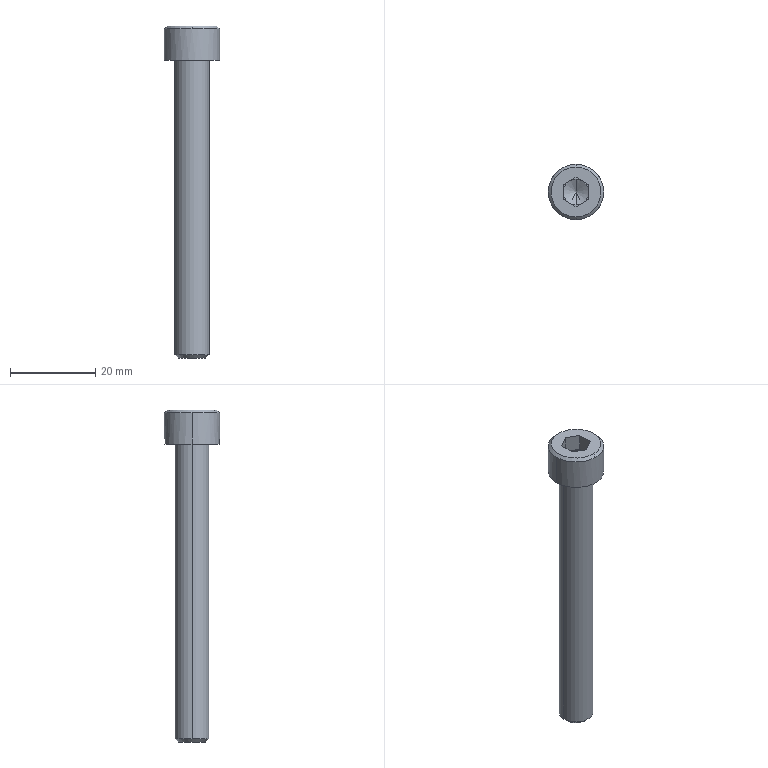Part | SolidWorks | features BaseBody 1 | 1 solid | 25 faces | box 13 x 13 x 78 mm | volume 4424 mm3 | plane 15 | cone 6 | cylinder 4 | commonest cylinder face diameters 8 x2 13 x2
STEP:
#1=CARTESIAN_POINT('',(4.,0.,-69.233));
#2=VERTEX_POINT('',#1);
#3=CARTESIAN_POINT('',(-4.,0.,-69.233));
#4=VERTEX_POINT('',#3);
#5=CARTESIAN_POINT('',(0.,0.,-69.233));
#6=DIRECTION('',(0.,0.,1.));
#7=DIRECTION('',(1.,0.,0.));
#8=AXIS2_PLACEMENT_3D('',#5,#6,#7);
#9=CIRCLE('',#8,4.);
#10=EDGE_CURVE('',#2,#4,#9,.T.);
#11=ORIENTED_EDGE('',*,*,#10,.T.);
#12=CARTESIAN_POINT('',(-4.,0.,0.));
#13=VERTEX_POINT('',#12);
#14=CARTESIAN_POINT('',(-4.,0.,-115.));
#15=DIRECTION('',(0.,0.,1.));
#16=VECTOR('',#15,1000.);
#17=LINE('',#14,#16);
#18=EDGE_CURVE('',#4,#13,#17,.T.);
#19=ORIENTED_EDGE('',*,*,#18,.T.);
#20=CARTESIAN_POINT('',(4.,0.,0.));
#21=VERTEX_POINT('',#20);
#22=CARTESIAN_POINT('',(0.,0.,0.));
#23=DIRECTION('',(0.,0.,-1.));
#24=DIRECTION('',(1.,0.,0.));
#25=AXIS2_PLACEMENT_3D('',#22,#23,#24);
#26=CIRCLE('',#25,4.);
#27=EDGE_CURVE('',#13,#21,#26,.T.);
#28=ORIENTED_EDGE('',*,*,#27,.T.);
#29=CARTESIAN_POINT('',(4.,0.,-115.));
#30=DIRECTION('',(0.,0.,1.));
#31=VECTOR('',#30,1000.);
#32=LINE('',#29,#31);
#33=EDGE_CURVE('',#2,#21,#32,.T.);
#34=ORIENTED_EDGE('',*,*,#33,.F.);
#35=EDGE_LOOP('',(#11,#19,#28,#34));
#36=FACE_OUTER_BOUND('',#35,.T.);
#37=CARTESIAN_POINT('',(0.,0.,-115.));
#38=DIRECTION('',(0.,0.,1.));
#39=DIRECTION('',(1.,0.,0.));
#40=AXIS2_PLACEMENT_3D('',#37,#38,#39);
#41=CYLINDRICAL_SURFACE('',#40,4.);
#42=ADVANCED_FACE('',(#36),#41,.T.);
#43=CARTESIAN_POINT('',(3.233,0.,-70.));
#44=VERTEX_POINT('',#43);
#45=CARTESIAN_POINT('',(-3.233,0.,-70.));
#46=VERTEX_POINT('',#45);
#47=CARTESIAN_POINT('',(0.,0.,-70.));
#48=DIRECTION('',(0.,0.,1.));
#49=DIRECTION('',(1.,0.,0.));
#50=AXIS2_PLACEMENT_3D('',#47,#48,#49);
#51=CIRCLE('',#50,3.233);
#52=EDGE_CURVE('',#44,#46,#51,.T.);
#53=ORIENTED_EDGE('',*,*,#52,.T.);
#54=CARTESIAN_POINT('',(-4.,0.,-69.233));
#55=DIRECTION('',(-0.7071,0.,0.7071));
#56=VECTOR('',#55,1000.);
#57=LINE('',#54,#56);
#58=EDGE_CURVE('',#46,#4,#57,.T.);
#59=ORIENTED_EDGE('',*,*,#58,.T.);
#60=ORIENTED_EDGE('',*,*,#10,.F.);
#61=CARTESIAN_POINT('',(4.,0.,-69.233));
#62=DIRECTION('',(0.7071,0.,0.7071));
#63=VECTOR('',#62,1000.);
#64=LINE('',#61,#63);
#65=EDGE_CURVE('',#44,#2,#64,.T.);
#66=ORIENTED_EDGE('',*,*,#65,.F.);
#67=EDGE_LOOP('',(#53,#59,#60,#66));
#68=FACE_OUTER_BOUND('',#67,.T.);
#69=CARTESIAN_POINT('',(0.,0.,-69.233));
#70=DIRECTION('',(0.,0.,1.));
#71=DIRECTION('',(1.,0.,0.));
#72=AXIS2_PLACEMENT_3D('',#69,#70,#71);
#73=CONICAL_SURFACE('',#72,4.,0.7854);
#74=ADVANCED_FACE('',(#68),#73,.T.);
#75=CARTESIAN_POINT('',(6.5,0.,0.));
#76=VERTEX_POINT('',#75);
#77=CARTESIAN_POINT('',(-6.5,0.,0.));
#78=VERTEX_POINT('',#77);
#79=CARTESIAN_POINT('',(0.,0.,0.));
#80=DIRECTION('',(0.,0.,1.));
#81=DIRECTION('',(1.,0.,0.));
#82=AXIS2_PLACEMENT_3D('',#79,#80,#81);
#83=CIRCLE('',#82,6.5);
#84=EDGE_CURVE('',#76,#78,#83,.T.);
#85=ORIENTED_EDGE('',*,*,#84,.T.);
#86=CARTESIAN_POINT('',(-6.5,0.,7.35));
#87=VERTEX_POINT('',#86);
#88=CARTESIAN_POINT('',(-6.5,0.,0.));
#89=DIRECTION('',(0.,0.,1.));
#90=VECTOR('',#89,1000.);
#91=LINE('',#88,#90);
#92=EDGE_CURVE('',#78,#87,#91,.T.);
#93=ORIENTED_EDGE('',*,*,#92,.T.);
#94=CARTESIAN_POINT('',(0.,6.5,7.35));
#95=VERTEX_POINT('',#94);
#96=CARTESIAN_POINT('',(0.,0.,7.35));
#97=DIRECTION('',(0.,0.,-1.));
#98=DIRECTION('',(1.,0.,0.));
#99=AXIS2_PLACEMENT_3D('',#96,#97,#98);
#100=CIRCLE('',#99,6.5);
#101=EDGE_CURVE('',#87,#95,#100,.T.);
#102=ORIENTED_EDGE('',*,*,#101,.T.);
#103=CARTESIAN_POINT('',(6.5,0.,7.35));
#104=VERTEX_POINT('',#103);
#105=CARTESIAN_POINT('',(0.,0.,7.35));
#106=DIRECTION('',(0.,0.,-1.));
#107=DIRECTION('',(1.,0.,0.));
#108=AXIS2_PLACEMENT_3D('',#105,#106,#107);
#109=CIRCLE('',#108,6.5);
#110=EDGE_CURVE('',#95,#104,#109,.T.);
#111=ORIENTED_EDGE('',*,*,#110,.T.);
#112=CARTESIAN_POINT('',(6.5,0.,0.));
#113=DIRECTION('',(0.,0.,1.));
#114=VECTOR('',#113,1000.);
#115=LINE('',#112,#114);
#116=EDGE_CURVE('',#76,#104,#115,.T.);
#117=ORIENTED_EDGE('',*,*,#116,.F.);
#118=EDGE_LOOP('',(#85,#93,#102,#111,#117));
#119=FACE_OUTER_BOUND('',#118,.T.);
#120=CARTESIAN_POINT('',(0.,0.,0.));
#121=DIRECTION('',(0.,0.,1.));
#122=DIRECTION('',(1.,0.,0.));
#123=AXIS2_PLACEMENT_3D('',#120,#121,#122);
#124=CYLINDRICAL_SURFACE('',#123,6.5);
#125=ADVANCED_FACE('',(#119),#124,.T.);
#126=CARTESIAN_POINT('',(0.,5.85,8.));
#127=VERTEX_POINT('',#126);
#128=CARTESIAN_POINT('',(0.,-5.85,8.));
#129=VERTEX_POINT('',#128);
#130=CARTESIAN_POINT('',(0.,0.,8.));
#131=DIRECTION('',(0.,0.,-1.));
#132=DIRECTION('',(0.,1.,0.));
#133=AXIS2_PLACEMENT_3D('',#130,#131,#132);
#134=CIRCLE('',#133,5.85);
#135=EDGE_CURVE('',#127,#129,#134,.T.);
#136=ORIENTED_EDGE('',*,*,#135,.T.);
#137=CARTESIAN_POINT('',(0.,-6.5,7.35));
#138=VERTEX_POINT('',#137);
#139=CARTESIAN_POINT('',(0.,-6.5,7.35));
#140=DIRECTION('',(0.,-0.7071,-0.7071));
#141=VECTOR('',#140,1000.);
#142=LINE('',#139,#141);
#143=EDGE_CURVE('',#129,#138,#142,.T.);
#144=ORIENTED_EDGE('',*,*,#143,.T.);
#145=CARTESIAN_POINT('',(0.,0.,7.35));
#146=DIRECTION('',(0.,0.,-1.));
#147=DIRECTION('',(1.,0.,0.));
#148=AXIS2_PLACEMENT_3D('',#145,#146,#147);
#149=CIRCLE('',#148,6.5);
#150=EDGE_CURVE('',#104,#138,#149,.T.);
#151=ORIENTED_EDGE('',*,*,#150,.F.);
#152=ORIENTED_EDGE('',*,*,#110,.F.);
#153=CARTESIAN_POINT('',(0.,6.5,7.35));
#154=DIRECTION('',(0.,0.7071,-0.7071));
#155=VECTOR('',#154,1000.);
#156=LINE('',#153,#155);
#157=EDGE_CURVE('',#127,#95,#156,.T.);
#158=ORIENTED_EDGE('',*,*,#157,.F.);
#159=EDGE_LOOP('',(#136,#144,#151,#152,#158));
#160=FACE_OUTER_BOUND('',#159,.T.);
#161=CARTESIAN_POINT('',(0.,0.,7.35));
#162=DIRECTION('',(0.,0.,-1.));
#163=DIRECTION('',(0.,1.,0.));
#164=AXIS2_PLACEMENT_3D('',#161,#162,#163);
#165=CONICAL_SURFACE('',#164,6.5,0.7854);
#166=ADVANCED_FACE('',(#160),#165,.T.);
#167=CARTESIAN_POINT('',(0.,0.,2.268));
#168=VERTEX_POINT('',#167);
#169=CARTESIAN_POINT('',(0.,-3.,4.));
#170=VERTEX_POINT('',#169);
#171=CARTESIAN_POINT('',(0.,-3.,4.));
#172=DIRECTION('',(0.,-0.866,0.5));
#173=VECTOR('',#172,1000.);
#174=LINE('',#171,#173);
#175=EDGE_CURVE('',#168,#170,#174,.T.);
#176=ORIENTED_EDGE('',*,*,#175,.F.);
#177=CARTESIAN_POINT('',(0.,3.,4.));
#178=VERTEX_POINT('',#177);
#179=CARTESIAN_POINT('',(0.,3.,4.));
#180=DIRECTION('',(0.,0.866,0.5));
#181=VECTOR('',#180,1000.);
#182=LINE('',#179,#181);
#183=EDGE_CURVE('',#168,#178,#182,.T.);
#184=ORIENTED_EDGE('',*,*,#183,.T.);
#185=CARTESIAN_POINT('',(-1.5,2.598,4.));
#186=VERTEX_POINT('',#185);
#187=CARTESIAN_POINT('',(0.,0.,4.));
#188=DIRECTION('',(0.,0.,-1.));
#189=DIRECTION('',(0.,-1.,0.));
#190=AXIS2_PLACEMENT_3D('',#187,#188,#189);
#191=CIRCLE('',#190,3.);
#192=EDGE_CURVE('',#186,#178,#191,.T.);
#193=ORIENTED_EDGE('',*,*,#192,.F.);
#194=CARTESIAN_POINT('',(-3.,0.,4.));
#195=VERTEX_POINT('',#194);
#196=CARTESIAN_POINT('',(0.,0.,4.));
#197=DIRECTION('',(0.,0.,-1.));
#198=DIRECTION('',(0.,-1.,0.));
#199=AXIS2_PLACEMENT_3D('',#196,#197,#198);
#200=CIRCLE('',#199,3.);
#201=EDGE_CURVE('',#195,#186,#200,.T.);
#202=ORIENTED_EDGE('',*,*,#201,.F.);
#203=CARTESIAN_POINT('',(-1.5,-2.598,4.));
#204=VERTEX_POINT('',#203);
#205=CARTESIAN_POINT('',(0.,0.,4.));
#206=DIRECTION('',(0.,0.,-1.));
#207=DIRECTION('',(0.,-1.,0.));
#208=AXIS2_PLACEMENT_3D('',#205,#206,#207);
#209=CIRCLE('',#208,3.);
#210=EDGE_CURVE('',#204,#195,#209,.T.);
#211=ORIENTED_EDGE('',*,*,#210,.F.);
#212=CARTESIAN_POINT('',(0.,0.,4.));
#213=DIRECTION('',(0.,0.,-1.));
#214=DIRECTION('',(0.,-1.,0.));
#215=AXIS2_PLACEMENT_3D('',#212,#213,#214);
#216=CIRCLE('',#215,3.);
#217=EDGE_CURVE('',#170,#204,#216,.T.);
#218=ORIENTED_EDGE('',*,*,#217,.F.);
#219=EDGE_LOOP('',(#176,#184,#193,#202,#211,#218));
#220=FACE_OUTER_BOUND('',#219,.T.);
#221=CARTESIAN_POINT('',(0.,0.,4.));
#222=DIRECTION('',(0.,0.,1.));
#223=DIRECTION('',(0.,-1.,0.));
#224=AXIS2_PLACEMENT_3D('',#221,#222,#223);
#225=CONICAL_SURFACE('',#224,3.,1.047);
#226=ADVANCED_FACE('',(#220),#225,.F.);
#227=ORIENTED_EDGE('',*,*,#18,.F.);
#228=CARTESIAN_POINT('',(0.,0.,-69.233));
#229=DIRECTION('',(0.,0.,1.));
#230=DIRECTION('',(1.,0.,0.));
#231=AXIS2_PLACEMENT_3D('',#228,#229,#230);
#232=CIRCLE('',#231,4.);
#233=EDGE_CURVE('',#4,#2,#232,.T.);
#234=ORIENTED_EDGE('',*,*,#233,.T.);
#235=ORIENTED_EDGE('',*,*,#33,.T.);
#236=CARTESIAN_POINT('',(0.,0.,0.));
#237=DIRECTION('',(0.,0.,-1.));
#238=DIRECTION('',(1.,0.,0.));
#239=AXIS2_PLACEMENT_3D('',#236,#237,#238);
#240=CIRCLE('',#239,4.);
#241=EDGE_CURVE('',#21,#13,#240,.T.);
#242=ORIENTED_EDGE('',*,*,#241,.T.);
#243=EDGE_LOOP('',(#227,#234,#235,#242));
#244=FACE_OUTER_BOUND('',#243,.T.);
#245=CARTESIAN_POINT('',(0.,0.,-115.));
#246=DIRECTION('',(0.,0.,1.));
#247=DIRECTION('',(1.,0.,0.));
#248=AXIS2_PLACEMENT_3D('',#245,#246,#247);
#249=CYLINDRICAL_SURFACE('',#248,4.);
#250=ADVANCED_FACE('',(#244),#249,.T.);
#251=ORIENTED_EDGE('',*,*,#84,.F.);
#252=CARTESIAN_POINT('',(0.,0.,0.));
#253=DIRECTION('',(0.,0.,1.));
#254=DIRECTION('',(1.,0.,0.));
#255=AXIS2_PLACEMENT_3D('',#252,#253,#254);
#256=CIRCLE('',#255,6.5);
#257=EDGE_CURVE('',#78,#76,#256,.T.);
#258=ORIENTED_EDGE('',*,*,#257,.F.);
#259=EDGE_LOOP('',(#251,#258));
#260=FACE_OUTER_BOUND('',#259,.T.);
#261=ORIENTED_EDGE('',*,*,#241,.F.);
#262=ORIENTED_EDGE('',*,*,#27,.F.);
#263=EDGE_LOOP('',(#261,#262));
#264=FACE_BOUND('',#263,.T.);
#265=CARTESIAN_POINT('',(0.,6.5,0.));
#266=DIRECTION('',(0.,0.,1.));
#267=DIRECTION('',(1.,0.,0.));
#268=AXIS2_PLACEMENT_3D('',#265,#266,#267);
#269=PLANE('',#268);
#270=ADVANCED_FACE('',(#260,#264),#269,.F.);
#271=ORIENTED_EDGE('',*,*,#58,.F.);
#272=CARTESIAN_POINT('',(0.,0.,-70.));
#273=DIRECTION('',(0.,0.,1.));
#274=DIRECTION('',(1.,0.,0.));
#275=AXIS2_PLACEMENT_3D('',#272,#273,#274);
#276=CIRCLE('',#275,3.233);
#277=EDGE_CURVE('',#46,#44,#276,.T.);
#278=ORIENTED_EDGE('',*,*,#277,.T.);
#279=ORIENTED_EDGE('',*,*,#65,.T.);
#280=ORIENTED_EDGE('',*,*,#233,.F.);
#281=EDGE_LOOP('',(#271,#278,#279,#280));
#282=FACE_OUTER_BOUND('',#281,.T.);
#283=CARTESIAN_POINT('',(0.,0.,-69.233));
#284=DIRECTION('',(0.,0.,1.));
#285=DIRECTION('',(1.,0.,0.));
#286=AXIS2_PLACEMENT_3D('',#283,#284,#285);
#287=CONICAL_SURFACE('',#286,4.,0.7854);
#288=ADVANCED_FACE('',(#282),#287,.T.);
#289=ORIENTED_EDGE('',*,*,#92,.F.);
#290=ORIENTED_EDGE('',*,*,#257,.T.);
#291=ORIENTED_EDGE('',*,*,#116,.T.);
#292=ORIENTED_EDGE('',*,*,#150,.T.);
#293=CARTESIAN_POINT('',(0.,0.,7.35));
#294=DIRECTION('',(0.,0.,-1.));
#295=DIRECTION('',(1.,0.,0.));
#296=AXIS2_PLACEMENT_3D('',#293,#294,#295);
#297=CIRCLE('',#296,6.5);
#298=EDGE_CURVE('',#138,#87,#297,.T.);
#299=ORIENTED_EDGE('',*,*,#298,.T.);
#300=EDGE_LOOP('',(#289,#290,#291,#292,#299));
#301=FACE_OUTER_BOUND('',#300,.T.);
#302=CARTESIAN_POINT('',(0.,0.,0.));
#303=DIRECTION('',(0.,0.,1.));
#304=DIRECTION('',(1.,0.,0.));
#305=AXIS2_PLACEMENT_3D('',#302,#303,#304);
#306=CYLINDRICAL_SURFACE('',#305,6.5);
#307=ADVANCED_FACE('',(#301),#306,.T.);
#308=ORIENTED_EDGE('',*,*,#52,.F.);
#309=ORIENTED_EDGE('',*,*,#277,.F.);
#310=EDGE_LOOP('',(#308,#309));
#311=FACE_OUTER_BOUND('',#310,.T.);
#312=CARTESIAN_POINT('',(0.,3.233,-70.));
#313=DIRECTION('',(0.,0.,1.));
#314=DIRECTION('',(1.,0.,0.));
#315=AXIS2_PLACEMENT_3D('',#312,#313,#314);
#316=PLANE('',#315);
#317=ADVANCED_FACE('',(#311),#316,.F.);
#318=ORIENTED_EDGE('',*,*,#143,.F.);
#319=CARTESIAN_POINT('',(0.,0.,8.));
#320=DIRECTION('',(0.,0.,-1.));
#321=DIRECTION('',(0.,1.,0.));
#322=AXIS2_PLACEMENT_3D('',#319,#320,#321);
#323=CIRCLE('',#322,5.85);
#324=EDGE_CURVE('',#129,#127,#323,.T.);
#325=ORIENTED_EDGE('',*,*,#324,.T.);
#326=ORIENTED_EDGE('',*,*,#157,.T.);
#327=ORIENTED_EDGE('',*,*,#101,.F.);
#328=ORIENTED_EDGE('',*,*,#298,.F.);
#329=EDGE_LOOP('',(#318,#325,#326,#327,#328));
#330=FACE_OUTER_BOUND('',#329,.T.);
#331=CARTESIAN_POINT('',(0.,0.,7.35));
#332=DIRECTION('',(0.,0.,-1.));
#333=DIRECTION('',(0.,1.,0.));
#334=AXIS2_PLACEMENT_3D('',#331,#332,#333);
#335=CONICAL_SURFACE('',#334,6.5,0.7854);
#336=ADVANCED_FACE('',(#330),#335,.T.);
#337=CARTESIAN_POINT('',(-3.,-1.732,8.));
#338=VERTEX_POINT('',#337);
#339=CARTESIAN_POINT('',(0.,-3.464,8.));
#340=VERTEX_POINT('',#339);
#341=CARTESIAN_POINT('',(-3.,-1.732,8.));
#342=DIRECTION('',(0.866,-0.5,0.));
#343=VECTOR('',#342,1000.);
#344=LINE('',#341,#343);
#345=EDGE_CURVE('',#338,#340,#344,.T.);
#346=ORIENTED_EDGE('',*,*,#345,.F.);
#347=CARTESIAN_POINT('',(-3.,1.732,8.));
#348=VERTEX_POINT('',#347);
#349=CARTESIAN_POINT('',(-3.,0.,8.));
#350=DIRECTION('',(0.,-1.,0.));
#351=VECTOR('',#350,1000.);
#352=LINE('',#349,#351);
#353=EDGE_CURVE('',#348,#338,#352,.T.);
#354=ORIENTED_EDGE('',*,*,#353,.F.);
#355=CARTESIAN_POINT('',(0.,3.464,8.));
#356=VERTEX_POINT('',#355);
#357=CARTESIAN_POINT('',(0.,3.464,8.));
#358=DIRECTION('',(-0.866,-0.5,0.));
#359=VECTOR('',#358,1000.);
#360=LINE('',#357,#359);
#361=EDGE_CURVE('',#356,#348,#360,.T.);
#362=ORIENTED_EDGE('',*,*,#361,.F.);
#363=CARTESIAN_POINT('',(3.,1.732,8.));
#364=VERTEX_POINT('',#363);
#365=CARTESIAN_POINT('',(3.,1.732,8.));
#366=DIRECTION('',(-0.866,0.5,0.));
#367=VECTOR('',#366,1000.);
#368=LINE('',#365,#367);
#369=EDGE_CURVE('',#364,#356,#368,.T.);
#370=ORIENTED_EDGE('',*,*,#369,.F.);
#371=CARTESIAN_POINT('',(3.,-1.732,8.));
#372=VERTEX_POINT('',#371);
#373=CARTESIAN_POINT('',(3.,0.,8.));
#374=DIRECTION('',(0.,1.,0.));
#375=VECTOR('',#374,1000.);
#376=LINE('',#373,#375);
#377=EDGE_CURVE('',#372,#364,#376,.T.);
#378=ORIENTED_EDGE('',*,*,#377,.F.);
#379=CARTESIAN_POINT('',(0.,-3.464,8.));
#380=DIRECTION('',(0.866,0.5,0.));
#381=VECTOR('',#380,1000.);
#382=LINE('',#379,#381);
#383=EDGE_CURVE('',#340,#372,#382,.T.);
#384=ORIENTED_EDGE('',*,*,#383,.F.);
#385=EDGE_LOOP('',(#346,#354,#362,#370,#378,#384));
#386=FACE_BOUND('',#385,.T.);
#387=ORIENTED_EDGE('',*,*,#135,.F.);
#388=ORIENTED_EDGE('',*,*,#324,.F.);
#389=EDGE_LOOP('',(#387,#388));
#390=FACE_OUTER_BOUND('',#389,.T.);
#391=CARTESIAN_POINT('',(0.,0.,8.));
#392=DIRECTION('',(0.,0.,-1.));
#393=DIRECTION('',(-1.,0.,0.));
#394=AXIS2_PLACEMENT_3D('',#391,#392,#393);
#395=PLANE('',#394);
#396=ADVANCED_FACE('',(#386,#390),#395,.F.);
#397=CARTESIAN_POINT('',(3.,-1.732,4.));
#398=VERTEX_POINT('',#397);
#399=CARTESIAN_POINT('',(3.,-1.732,4.));
#400=DIRECTION('',(0.,0.,1.));
#401=VECTOR('',#400,1000.);
#402=LINE('',#399,#401);
#403=EDGE_CURVE('',#398,#372,#402,.T.);
#404=ORIENTED_EDGE('',*,*,#403,.F.);
#405=CARTESIAN_POINT('',(1.5,-2.598,4.));
#406=VERTEX_POINT('',#405);
#407=CARTESIAN_POINT('',(1.5,-2.598,4.));
#408=DIRECTION('',(0.866,0.5,0.));
#409=VECTOR('',#408,1000.);
#410=LINE('',#407,#409);
#411=EDGE_CURVE('',#406,#398,#410,.T.);
#412=ORIENTED_EDGE('',*,*,#411,.F.);
#413=CARTESIAN_POINT('',(0.,-3.464,4.));
#414=VERTEX_POINT('',#413);
#415=CARTESIAN_POINT('',(0.,-3.464,4.));
#416=DIRECTION('',(0.866,0.5,0.));
#417=VECTOR('',#416,1000.);
#418=LINE('',#415,#417);
#419=EDGE_CURVE('',#414,#406,#418,.T.);
#420=ORIENTED_EDGE('',*,*,#419,.F.);
#421=CARTESIAN_POINT('',(0.,-3.464,4.));
#422=DIRECTION('',(0.,0.,-1.));
#423=VECTOR('',#422,1000.);
#424=LINE('',#421,#423);
#425=EDGE_CURVE('',#340,#414,#424,.T.);
#426=ORIENTED_EDGE('',*,*,#425,.F.);
#427=ORIENTED_EDGE('',*,*,#383,.T.);
#428=EDGE_LOOP('',(#404,#412,#420,#426,#427));
#429=FACE_OUTER_BOUND('',#428,.T.);
#430=CARTESIAN_POINT('',(0.,-3.464,4.));
#431=DIRECTION('',(0.5,-0.866,0.));
#432=DIRECTION('',(0.866,0.5,0.));
#433=AXIS2_PLACEMENT_3D('',#430,#431,#432);
#434=PLANE('',#433);
#435=ADVANCED_FACE('',(#429),#434,.F.);
#436=ORIENTED_EDGE('',*,*,#425,.T.);
#437=CARTESIAN_POINT('',(-1.5,-2.598,4.));
#438=DIRECTION('',(0.866,-0.5,0.));
#439=VECTOR('',#438,1000.);
#440=LINE('',#437,#439);
#441=EDGE_CURVE('',#204,#414,#440,.T.);
#442=ORIENTED_EDGE('',*,*,#441,.F.);
#443=CARTESIAN_POINT('',(-3.,-1.732,4.));
#444=VERTEX_POINT('',#443);
#445=CARTESIAN_POINT('',(-3.,-1.732,4.));
#446=DIRECTION('',(0.866,-0.5,0.));
#447=VECTOR('',#446,1000.);
#448=LINE('',#445,#447);
#449=EDGE_CURVE('',#444,#204,#448,.T.);
#450=ORIENTED_EDGE('',*,*,#449,.F.);
#451=CARTESIAN_POINT('',(-3.,-1.732,4.));
#452=DIRECTION('',(0.,0.,-1.));
#453=VECTOR('',#452,1000.);
#454=LINE('',#451,#453);
#455=EDGE_CURVE('',#338,#444,#454,.T.);
#456=ORIENTED_EDGE('',*,*,#455,.F.);
#457=ORIENTED_EDGE('',*,*,#345,.T.);
#458=EDGE_LOOP('',(#436,#442,#450,#456,#457));
#459=FACE_OUTER_BOUND('',#458,.T.);
#460=CARTESIAN_POINT('',(-3.,-1.732,4.));
#461=DIRECTION('',(-0.5,-0.866,0.));
#462=DIRECTION('',(0.866,-0.5,0.));
#463=AXIS2_PLACEMENT_3D('',#460,#461,#462);
#464=PLANE('',#463);
#465=ADVANCED_FACE('',(#459),#464,.F.);
#466=ORIENTED_EDGE('',*,*,#455,.T.);
#467=CARTESIAN_POINT('',(-3.,0.,4.));
#468=DIRECTION('',(0.,-1.,0.));
#469=VECTOR('',#468,1000.);
#470=LINE('',#467,#469);
#471=EDGE_CURVE('',#195,#444,#470,.T.);
#472=ORIENTED_EDGE('',*,*,#471,.F.);
#473=CARTESIAN_POINT('',(-3.,1.732,4.));
#474=VERTEX_POINT('',#473);
#475=CARTESIAN_POINT('',(-3.,0.,4.));
#476=DIRECTION('',(0.,-1.,0.));
#477=VECTOR('',#476,1000.);
#478=LINE('',#475,#477);
#479=EDGE_CURVE('',#474,#195,#478,.T.);
#480=ORIENTED_EDGE('',*,*,#479,.F.);
#481=CARTESIAN_POINT('',(-3.,1.732,4.));
#482=DIRECTION('',(0.,0.,-1.));
#483=VECTOR('',#482,1000.);
#484=LINE('',#481,#483);
#485=EDGE_CURVE('',#348,#474,#484,.T.);
#486=ORIENTED_EDGE('',*,*,#485,.F.);
#487=ORIENTED_EDGE('',*,*,#353,.T.);
#488=EDGE_LOOP('',(#466,#472,#480,#486,#487));
#489=FACE_OUTER_BOUND('',#488,.T.);
#490=CARTESIAN_POINT('',(-3.,1.732,4.));
#491=DIRECTION('',(-1.,0.,0.));
#492=DIRECTION('',(0.,0.,1.));
#493=AXIS2_PLACEMENT_3D('',#490,#491,#492);
#494=PLANE('',#493);
#495=ADVANCED_FACE('',(#489),#494,.F.);
#496=ORIENTED_EDGE('',*,*,#485,.T.);
#497=CARTESIAN_POINT('',(-1.5,2.598,4.));
#498=DIRECTION('',(-0.866,-0.5,0.));
#499=VECTOR('',#498,1000.);
#500=LINE('',#497,#499);
#501=EDGE_CURVE('',#186,#474,#500,.T.);
#502=ORIENTED_EDGE('',*,*,#501,.F.);
#503=CARTESIAN_POINT('',(0.,3.464,4.));
#504=VERTEX_POINT('',#503);
#505=CARTESIAN_POINT('',(0.,3.464,4.));
#506=DIRECTION('',(-0.866,-0.5,0.));
#507=VECTOR('',#506,1000.);
#508=LINE('',#505,#507);
#509=EDGE_CURVE('',#504,#186,#508,.T.);
#510=ORIENTED_EDGE('',*,*,#509,.F.);
#511=CARTESIAN_POINT('',(0.,3.464,4.));
#512=DIRECTION('',(0.,0.,-1.));
#513=VECTOR('',#512,1000.);
#514=LINE('',#511,#513);
#515=EDGE_CURVE('',#356,#504,#514,.T.);
#516=ORIENTED_EDGE('',*,*,#515,.F.);
#517=ORIENTED_EDGE('',*,*,#361,.T.);
#518=EDGE_LOOP('',(#496,#502,#510,#516,#517));
#519=FACE_OUTER_BOUND('',#518,.T.);
#520=CARTESIAN_POINT('',(0.,3.464,4.));
#521=DIRECTION('',(-0.5,0.866,0.));
#522=DIRECTION('',(-0.866,-0.5,0.));
#523=AXIS2_PLACEMENT_3D('',#520,#521,#522);
#524=PLANE('',#523);
#525=ADVANCED_FACE('',(#519),#524,.F.);
#526=ORIENTED_EDGE('',*,*,#515,.T.);
#527=CARTESIAN_POINT('',(1.5,2.598,4.));
#528=VERTEX_POINT('',#527);
#529=CARTESIAN_POINT('',(1.5,2.598,4.));
#530=DIRECTION('',(-0.866,0.5,0.));
#531=VECTOR('',#530,1000.);
#532=LINE('',#529,#531);
#533=EDGE_CURVE('',#528,#504,#532,.T.);
#534=ORIENTED_EDGE('',*,*,#533,.F.);
#535=CARTESIAN_POINT('',(3.,1.732,4.));
#536=VERTEX_POINT('',#535);
#537=CARTESIAN_POINT('',(3.,1.732,4.));
#538=DIRECTION('',(-0.866,0.5,0.));
#539=VECTOR('',#538,1000.);
#540=LINE('',#537,#539);
#541=EDGE_CURVE('',#536,#528,#540,.T.);
#542=ORIENTED_EDGE('',*,*,#541,.F.);
#543=CARTESIAN_POINT('',(3.,1.732,4.));
#544=DIRECTION('',(0.,0.,-1.));
#545=VECTOR('',#544,1000.);
#546=LINE('',#543,#545);
#547=EDGE_CURVE('',#364,#536,#546,.T.);
#548=ORIENTED_EDGE('',*,*,#547,.F.);
#549=ORIENTED_EDGE('',*,*,#369,.T.);
#550=EDGE_LOOP('',(#526,#534,#542,#548,#549));
#551=FACE_OUTER_BOUND('',#550,.T.);
#552=CARTESIAN_POINT('',(3.,1.732,4.));
#553=DIRECTION('',(0.5,0.866,0.));
#554=DIRECTION('',(-0.866,0.5,0.));
#555=AXIS2_PLACEMENT_3D('',#552,#553,#554);
#556=PLANE('',#555);
#557=ADVANCED_FACE('',(#551),#556,.F.);
#558=ORIENTED_EDGE('',*,*,#547,.T.);
#559=CARTESIAN_POINT('',(3.,0.,4.));
#560=VERTEX_POINT('',#559);
#561=CARTESIAN_POINT('',(3.,-1.732,4.));
#562=DIRECTION('',(0.,1.,0.));
#563=VECTOR('',#562,1000.);
#564=LINE('',#561,#563);
#565=EDGE_CURVE('',#560,#536,#564,.T.);
#566=ORIENTED_EDGE('',*,*,#565,.F.);
#567=CARTESIAN_POINT('',(3.,0.,4.));
#568=DIRECTION('',(0.,1.,0.));
#569=VECTOR('',#568,1000.);
#570=LINE('',#567,#569);
#571=EDGE_CURVE('',#398,#560,#570,.T.);
#572=ORIENTED_EDGE('',*,*,#571,.F.);
#573=ORIENTED_EDGE('',*,*,#403,.T.);
#574=ORIENTED_EDGE('',*,*,#377,.T.);
#575=EDGE_LOOP('',(#558,#566,#572,#573,#574));
#576=FACE_OUTER_BOUND('',#575,.T.);
#577=CARTESIAN_POINT('',(3.,-1.732,4.));
#578=DIRECTION('',(1.,0.,0.));
#579=DIRECTION('',(0.,0.,-1.));
#580=AXIS2_PLACEMENT_3D('',#577,#578,#579);
#581=PLANE('',#580);
#582=ADVANCED_FACE('',(#576),#581,.F.);
#583=CARTESIAN_POINT('',(0.,0.,4.));
#584=DIRECTION('',(0.,0.,-1.));
#585=DIRECTION('',(0.,-1.,0.));
#586=AXIS2_PLACEMENT_3D('',#583,#584,#585);
#587=CIRCLE('',#586,3.);
#588=EDGE_CURVE('',#528,#560,#587,.T.);
#589=ORIENTED_EDGE('',*,*,#588,.T.);
#590=ORIENTED_EDGE('',*,*,#565,.T.);
#591=ORIENTED_EDGE('',*,*,#541,.T.);
#592=EDGE_LOOP('',(#589,#590,#591));
#593=FACE_OUTER_BOUND('',#592,.T.);
#594=CARTESIAN_POINT('',(0.,0.,4.));
#595=DIRECTION('',(0.,0.,1.));
#596=DIRECTION('',(1.,0.,0.));
#597=AXIS2_PLACEMENT_3D('',#594,#595,#596);
#598=PLANE('',#597);
#599=ADVANCED_FACE('',(#593),#598,.T.);
#600=ORIENTED_EDGE('',*,*,#183,.F.);
#601=ORIENTED_EDGE('',*,*,#175,.T.);
#602=CARTESIAN_POINT('',(0.,0.,4.));
#603=DIRECTION('',(0.,0.,-1.));
#604=DIRECTION('',(0.,-1.,0.));
#605=AXIS2_PLACEMENT_3D('',#602,#603,#604);
#606=CIRCLE('',#605,3.);
#607=EDGE_CURVE('',#406,#170,#606,.T.);
#608=ORIENTED_EDGE('',*,*,#607,.F.);
#609=CARTESIAN_POINT('',(0.,0.,4.));
#610=DIRECTION('',(0.,0.,-1.));
#611=DIRECTION('',(0.,-1.,0.));
#612=AXIS2_PLACEMENT_3D('',#609,#610,#611);
#613=CIRCLE('',#612,3.);
#614=EDGE_CURVE('',#560,#406,#613,.T.);
#615=ORIENTED_EDGE('',*,*,#614,.F.);
#616=ORIENTED_EDGE('',*,*,#588,.F.);
#617=CARTESIAN_POINT('',(0.,0.,4.));
#618=DIRECTION('',(0.,0.,-1.));
#619=DIRECTION('',(0.,-1.,0.));
#620=AXIS2_PLACEMENT_3D('',#617,#618,#619);
#621=CIRCLE('',#620,3.);
#622=EDGE_CURVE('',#178,#528,#621,.T.);
#623=ORIENTED_EDGE('',*,*,#622,.F.);
#624=EDGE_LOOP('',(#600,#601,#608,#615,#616,#623));
#625=FACE_OUTER_BOUND('',#624,.T.);
#626=CARTESIAN_POINT('',(0.,0.,4.));
#627=DIRECTION('',(0.,0.,1.));
#628=DIRECTION('',(0.,-1.,0.));
#629=AXIS2_PLACEMENT_3D('',#626,#627,#628);
#630=CONICAL_SURFACE('',#629,3.,1.047);
#631=ADVANCED_FACE('',(#625),#630,.F.);
#632=ORIENTED_EDGE('',*,*,#192,.T.);
#633=ORIENTED_EDGE('',*,*,#622,.T.);
#634=ORIENTED_EDGE('',*,*,#533,.T.);
#635=ORIENTED_EDGE('',*,*,#509,.T.);
#636=EDGE_LOOP('',(#632,#633,#634,#635));
#637=FACE_OUTER_BOUND('',#636,.T.);
#638=CARTESIAN_POINT('',(0.,0.,4.));
#639=DIRECTION('',(0.,0.,1.));
#640=DIRECTION('',(1.,0.,0.));
#641=AXIS2_PLACEMENT_3D('',#638,#639,#640);
#642=PLANE('',#641);
#643=ADVANCED_FACE('',(#637),#642,.T.);
#644=ORIENTED_EDGE('',*,*,#201,.T.);
#645=ORIENTED_EDGE('',*,*,#501,.T.);
#646=ORIENTED_EDGE('',*,*,#479,.T.);
#647=EDGE_LOOP('',(#644,#645,#646));
#648=FACE_OUTER_BOUND('',#647,.T.);
#649=CARTESIAN_POINT('',(0.,0.,4.));
#650=DIRECTION('',(0.,0.,1.));
#651=DIRECTION('',(1.,0.,0.));
#652=AXIS2_PLACEMENT_3D('',#649,#650,#651);
#653=PLANE('',#652);
#654=ADVANCED_FACE('',(#648),#653,.T.);
#655=ORIENTED_EDGE('',*,*,#210,.T.);
#656=ORIENTED_EDGE('',*,*,#471,.T.);
#657=ORIENTED_EDGE('',*,*,#449,.T.);
#658=EDGE_LOOP('',(#655,#656,#657));
#659=FACE_OUTER_BOUND('',#658,.T.);
#660=CARTESIAN_POINT('',(0.,0.,4.));
#661=DIRECTION('',(0.,0.,1.));
#662=DIRECTION('',(1.,0.,0.));
#663=AXIS2_PLACEMENT_3D('',#660,#661,#662);
#664=PLANE('',#663);
#665=ADVANCED_FACE('',(#659),#664,.T.);
#666=ORIENTED_EDGE('',*,*,#607,.T.);
#667=ORIENTED_EDGE('',*,*,#217,.T.);
#668=ORIENTED_EDGE('',*,*,#441,.T.);
#669=ORIENTED_EDGE('',*,*,#419,.T.);
#670=EDGE_LOOP('',(#666,#667,#668,#669));
#671=FACE_OUTER_BOUND('',#670,.T.);
#672=CARTESIAN_POINT('',(0.,0.,4.));
#673=DIRECTION('',(0.,0.,1.));
#674=DIRECTION('',(1.,0.,0.));
#675=AXIS2_PLACEMENT_3D('',#672,#673,#674);
#676=PLANE('',#675);
#677=ADVANCED_FACE('',(#671),#676,.T.);
#678=ORIENTED_EDGE('',*,*,#614,.T.);
#679=ORIENTED_EDGE('',*,*,#411,.T.);
#680=ORIENTED_EDGE('',*,*,#571,.T.);
#681=EDGE_LOOP('',(#678,#679,#680));
#682=FACE_OUTER_BOUND('',#681,.T.);
#683=CARTESIAN_POINT('',(0.,0.,4.));
#684=DIRECTION('',(0.,0.,1.));
#685=DIRECTION('',(1.,0.,0.));
#686=AXIS2_PLACEMENT_3D('',#683,#684,#685);
#687=PLANE('',#686);
#688=ADVANCED_FACE('',(#682),#687,.T.);
#689=CLOSED_SHELL('',(#42,#74,#125,#166,#226,#250,#270,#288,#307,#317,#336,#396,#435,#465,#495,#525,#557,#582,#599,#631,#643,#654,#665,#677,#688));
#690=MANIFOLD_SOLID_BREP('',#689);
#691=CARTESIAN_POINT('',(0.,0.,0.));
#692=DIRECTION('',(0.,0.,1.));
#693=DIRECTION('',(1.,0.,0.));
#694=AXIS2_PLACEMENT_3D('',#691,#692,#693);
#695=(LENGTH_UNIT()NAMED_UNIT(*)SI_UNIT(.MILLI.,.METRE.));
#696=UNCERTAINTY_MEASURE_WITH_UNIT(LENGTH_MEASURE(0.00001),#695,'','');
#697=(NAMED_UNIT(*)PLANE_ANGLE_UNIT()SI_UNIT($,.RADIAN.));
#698=(NAMED_UNIT(*)SI_UNIT($,.STERADIAN.)SOLID_ANGLE_UNIT());
#699=(GEOMETRIC_REPRESENTATION_CONTEXT(3)GLOBAL_UNCERTAINTY_ASSIGNED_CONTEXT((#696))GLOBAL_UNIT_ASSIGNED_CONTEXT((#695,#697,#698))REPRESENTATION_CONTEXT('',''));
#700=ADVANCED_BREP_SHAPE_REPRESENTATION('',(#690,#694),#699);